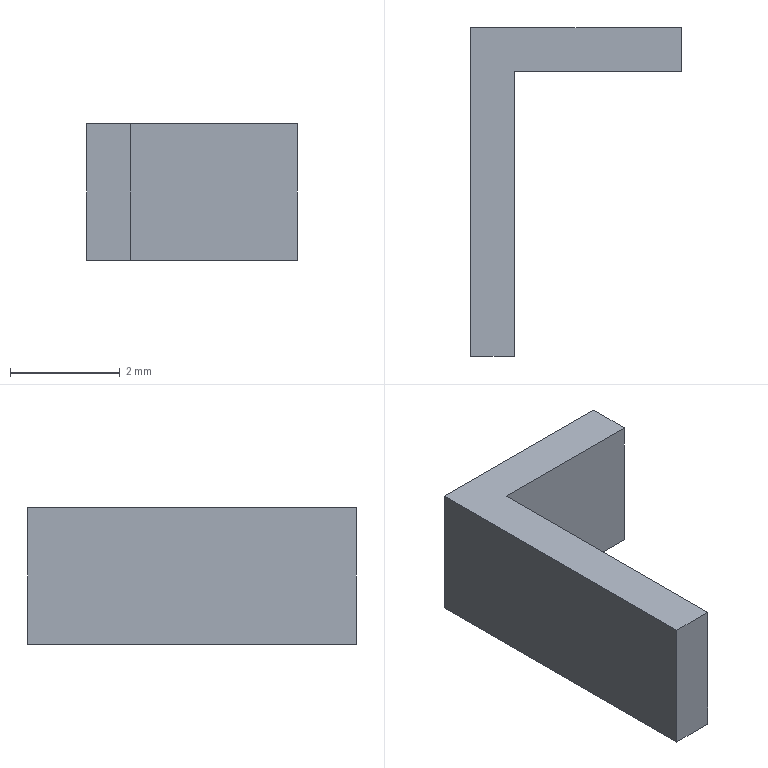Part | STEP file | lll_id1138_x_t | 1 solid | 8 faces | box 3.85 x 6 x 2.5 mm | volume 18.1 mm3 | plane 8
STEP:
#1=CARTESIAN_POINT('',(388.657,-103.274,2.35));
#2=VERTEX_POINT('',#1);
#3=CARTESIAN_POINT('',(387.857,-103.274,2.35));
#4=VERTEX_POINT('',#3);
#5=CARTESIAN_POINT('',(388.257,-103.274,2.35));
#6=DIRECTION('',(-1.,0.,0.));
#7=VECTOR('',#6,1.);
#8=LINE('',#5,#7);
#9=EDGE_CURVE('',#2,#4,#8,.T.);
#10=ORIENTED_EDGE('',*,*,#9,.T.);
#11=CARTESIAN_POINT('',(387.857,-103.274,-0.15));
#12=VERTEX_POINT('',#11);
#13=CARTESIAN_POINT('',(387.857,-103.274,-0.15));
#14=DIRECTION('',(0.,0.,1.));
#15=VECTOR('',#14,1.);
#16=LINE('',#13,#15);
#17=EDGE_CURVE('',#12,#4,#16,.T.);
#18=ORIENTED_EDGE('',*,*,#17,.F.);
#19=CARTESIAN_POINT('',(388.657,-103.274,-0.15));
#20=VERTEX_POINT('',#19);
#21=CARTESIAN_POINT('',(388.257,-103.274,-0.15));
#22=DIRECTION('',(-1.,0.,0.));
#23=VECTOR('',#22,1.);
#24=LINE('',#21,#23);
#25=EDGE_CURVE('',#20,#12,#24,.T.);
#26=ORIENTED_EDGE('',*,*,#25,.F.);
#27=CARTESIAN_POINT('',(388.657,-103.274,-0.15));
#28=DIRECTION('',(0.,0.,1.));
#29=VECTOR('',#28,1.);
#30=LINE('',#27,#29);
#31=EDGE_CURVE('',#20,#2,#30,.T.);
#32=ORIENTED_EDGE('',*,*,#31,.T.);
#33=EDGE_LOOP('',(#10,#18,#26,#32));
#34=FACE_OUTER_BOUND('',#33,.T.);
#35=CARTESIAN_POINT('',(388.657,-103.274,-0.15));
#36=DIRECTION('',(0.,1.,0.));
#37=DIRECTION('',(0.,0.,1.));
#38=AXIS2_PLACEMENT_3D('',#35,#36,#37);
#39=PLANE('',#38);
#40=ADVANCED_FACE('',(#34),#39,.F.);
#41=CARTESIAN_POINT('',(387.857,-97.274,2.35));
#42=VERTEX_POINT('',#41);
#43=CARTESIAN_POINT('',(387.857,-100.274,2.35));
#44=DIRECTION('',(0.,1.,0.));
#45=VECTOR('',#44,1.);
#46=LINE('',#43,#45);
#47=EDGE_CURVE('',#4,#42,#46,.T.);
#48=ORIENTED_EDGE('',*,*,#47,.T.);
#49=CARTESIAN_POINT('',(387.857,-97.274,-0.15));
#50=VERTEX_POINT('',#49);
#51=CARTESIAN_POINT('',(387.857,-97.274,-0.15));
#52=DIRECTION('',(0.,0.,1.));
#53=VECTOR('',#52,1.);
#54=LINE('',#51,#53);
#55=EDGE_CURVE('',#50,#42,#54,.T.);
#56=ORIENTED_EDGE('',*,*,#55,.F.);
#57=CARTESIAN_POINT('',(387.857,-100.274,-0.15));
#58=DIRECTION('',(0.,1.,0.));
#59=VECTOR('',#58,1.);
#60=LINE('',#57,#59);
#61=EDGE_CURVE('',#12,#50,#60,.T.);
#62=ORIENTED_EDGE('',*,*,#61,.F.);
#63=ORIENTED_EDGE('',*,*,#17,.T.);
#64=EDGE_LOOP('',(#48,#56,#62,#63));
#65=FACE_OUTER_BOUND('',#64,.T.);
#66=CARTESIAN_POINT('',(387.857,-103.274,-0.15));
#67=DIRECTION('',(1.,0.,0.));
#68=DIRECTION('',(0.,0.,-1.));
#69=AXIS2_PLACEMENT_3D('',#66,#67,#68);
#70=PLANE('',#69);
#71=ADVANCED_FACE('',(#65),#70,.F.);
#72=CARTESIAN_POINT('',(391.707,-97.274,2.35));
#73=VERTEX_POINT('',#72);
#74=CARTESIAN_POINT('',(389.782,-97.274,2.35));
#75=DIRECTION('',(1.,0.,0.));
#76=VECTOR('',#75,1.);
#77=LINE('',#74,#76);
#78=EDGE_CURVE('',#42,#73,#77,.T.);
#79=ORIENTED_EDGE('',*,*,#78,.T.);
#80=CARTESIAN_POINT('',(391.707,-97.274,-0.15));
#81=VERTEX_POINT('',#80);
#82=CARTESIAN_POINT('',(391.707,-97.274,-0.15));
#83=DIRECTION('',(0.,0.,1.));
#84=VECTOR('',#83,1.);
#85=LINE('',#82,#84);
#86=EDGE_CURVE('',#81,#73,#85,.T.);
#87=ORIENTED_EDGE('',*,*,#86,.F.);
#88=CARTESIAN_POINT('',(389.782,-97.274,-0.15));
#89=DIRECTION('',(1.,0.,0.));
#90=VECTOR('',#89,1.);
#91=LINE('',#88,#90);
#92=EDGE_CURVE('',#50,#81,#91,.T.);
#93=ORIENTED_EDGE('',*,*,#92,.F.);
#94=ORIENTED_EDGE('',*,*,#55,.T.);
#95=EDGE_LOOP('',(#79,#87,#93,#94));
#96=FACE_OUTER_BOUND('',#95,.T.);
#97=CARTESIAN_POINT('',(387.857,-97.274,-0.15));
#98=DIRECTION('',(0.,-1.,0.));
#99=DIRECTION('',(0.,0.,-1.));
#100=AXIS2_PLACEMENT_3D('',#97,#98,#99);
#101=PLANE('',#100);
#102=ADVANCED_FACE('',(#96),#101,.F.);
#103=CARTESIAN_POINT('',(391.707,-98.074,2.35));
#104=VERTEX_POINT('',#103);
#105=CARTESIAN_POINT('',(391.707,-97.674,2.35));
#106=DIRECTION('',(0.,-1.,0.));
#107=VECTOR('',#106,1.);
#108=LINE('',#105,#107);
#109=EDGE_CURVE('',#73,#104,#108,.T.);
#110=ORIENTED_EDGE('',*,*,#109,.T.);
#111=CARTESIAN_POINT('',(391.707,-98.074,-0.15));
#112=VERTEX_POINT('',#111);
#113=CARTESIAN_POINT('',(391.707,-98.074,-0.15));
#114=DIRECTION('',(0.,0.,1.));
#115=VECTOR('',#114,1.);
#116=LINE('',#113,#115);
#117=EDGE_CURVE('',#112,#104,#116,.T.);
#118=ORIENTED_EDGE('',*,*,#117,.F.);
#119=CARTESIAN_POINT('',(391.707,-97.674,-0.15));
#120=DIRECTION('',(0.,-1.,0.));
#121=VECTOR('',#120,1.);
#122=LINE('',#119,#121);
#123=EDGE_CURVE('',#81,#112,#122,.T.);
#124=ORIENTED_EDGE('',*,*,#123,.F.);
#125=ORIENTED_EDGE('',*,*,#86,.T.);
#126=EDGE_LOOP('',(#110,#118,#124,#125));
#127=FACE_OUTER_BOUND('',#126,.T.);
#128=CARTESIAN_POINT('',(391.707,-97.274,-0.15));
#129=DIRECTION('',(-1.,0.,0.));
#130=DIRECTION('',(0.,0.,1.));
#131=AXIS2_PLACEMENT_3D('',#128,#129,#130);
#132=PLANE('',#131);
#133=ADVANCED_FACE('',(#127),#132,.F.);
#134=CARTESIAN_POINT('',(388.657,-98.074,2.35));
#135=VERTEX_POINT('',#134);
#136=CARTESIAN_POINT('',(390.182,-98.074,2.35));
#137=DIRECTION('',(-1.,0.,0.));
#138=VECTOR('',#137,1.);
#139=LINE('',#136,#138);
#140=EDGE_CURVE('',#104,#135,#139,.T.);
#141=ORIENTED_EDGE('',*,*,#140,.T.);
#142=CARTESIAN_POINT('',(388.657,-98.074,-0.15));
#143=VERTEX_POINT('',#142);
#144=CARTESIAN_POINT('',(388.657,-98.074,-0.15));
#145=DIRECTION('',(0.,0.,1.));
#146=VECTOR('',#145,1.);
#147=LINE('',#144,#146);
#148=EDGE_CURVE('',#143,#135,#147,.T.);
#149=ORIENTED_EDGE('',*,*,#148,.F.);
#150=CARTESIAN_POINT('',(390.182,-98.074,-0.15));
#151=DIRECTION('',(-1.,0.,0.));
#152=VECTOR('',#151,1.);
#153=LINE('',#150,#152);
#154=EDGE_CURVE('',#112,#143,#153,.T.);
#155=ORIENTED_EDGE('',*,*,#154,.F.);
#156=ORIENTED_EDGE('',*,*,#117,.T.);
#157=EDGE_LOOP('',(#141,#149,#155,#156));
#158=FACE_OUTER_BOUND('',#157,.T.);
#159=CARTESIAN_POINT('',(391.707,-98.074,-0.15));
#160=DIRECTION('',(0.,1.,0.));
#161=DIRECTION('',(0.,0.,1.));
#162=AXIS2_PLACEMENT_3D('',#159,#160,#161);
#163=PLANE('',#162);
#164=ADVANCED_FACE('',(#158),#163,.F.);
#165=CARTESIAN_POINT('',(388.657,-100.674,2.35));
#166=DIRECTION('',(0.,-1.,0.));
#167=VECTOR('',#166,1.);
#168=LINE('',#165,#167);
#169=EDGE_CURVE('',#135,#2,#168,.T.);
#170=ORIENTED_EDGE('',*,*,#169,.T.);
#171=ORIENTED_EDGE('',*,*,#31,.F.);
#172=CARTESIAN_POINT('',(388.657,-100.674,-0.15));
#173=DIRECTION('',(0.,-1.,0.));
#174=VECTOR('',#173,1.);
#175=LINE('',#172,#174);
#176=EDGE_CURVE('',#143,#20,#175,.T.);
#177=ORIENTED_EDGE('',*,*,#176,.F.);
#178=ORIENTED_EDGE('',*,*,#148,.T.);
#179=EDGE_LOOP('',(#170,#171,#177,#178));
#180=FACE_OUTER_BOUND('',#179,.T.);
#181=CARTESIAN_POINT('',(388.657,-98.074,-0.15));
#182=DIRECTION('',(-1.,0.,0.));
#183=DIRECTION('',(0.,0.,1.));
#184=AXIS2_PLACEMENT_3D('',#181,#182,#183);
#185=PLANE('',#184);
#186=ADVANCED_FACE('',(#180),#185,.F.);
#187=ORIENTED_EDGE('',*,*,#25,.T.);
#188=ORIENTED_EDGE('',*,*,#61,.T.);
#189=ORIENTED_EDGE('',*,*,#92,.T.);
#190=ORIENTED_EDGE('',*,*,#123,.T.);
#191=ORIENTED_EDGE('',*,*,#154,.T.);
#192=ORIENTED_EDGE('',*,*,#176,.T.);
#193=EDGE_LOOP('',(#187,#188,#189,#190,#191,#192));
#194=FACE_OUTER_BOUND('',#193,.T.);
#195=CARTESIAN_POINT('',(388.257,-103.274,-0.15));
#196=DIRECTION('',(0.,0.,1.));
#197=DIRECTION('',(1.,0.,0.));
#198=AXIS2_PLACEMENT_3D('',#195,#196,#197);
#199=PLANE('',#198);
#200=ADVANCED_FACE('',(#194),#199,.F.);
#201=ORIENTED_EDGE('',*,*,#9,.F.);
#202=ORIENTED_EDGE('',*,*,#169,.F.);
#203=ORIENTED_EDGE('',*,*,#140,.F.);
#204=ORIENTED_EDGE('',*,*,#109,.F.);
#205=ORIENTED_EDGE('',*,*,#78,.F.);
#206=ORIENTED_EDGE('',*,*,#47,.F.);
#207=EDGE_LOOP('',(#201,#202,#203,#204,#205,#206));
#208=FACE_OUTER_BOUND('',#207,.T.);
#209=CARTESIAN_POINT('',(388.257,-103.274,2.35));
#210=DIRECTION('',(0.,0.,1.));
#211=DIRECTION('',(1.,0.,0.));
#212=AXIS2_PLACEMENT_3D('',#209,#210,#211);
#213=PLANE('',#212);
#214=ADVANCED_FACE('',(#208),#213,.T.);
#215=CLOSED_SHELL('',(#40,#71,#102,#133,#164,#186,#200,#214));
#216=MANIFOLD_SOLID_BREP('',#215);
#217=(LENGTH_UNIT()NAMED_UNIT(*)SI_UNIT(.MILLI.,.METRE.));
#218=UNCERTAINTY_MEASURE_WITH_UNIT(LENGTH_MEASURE(0.00002),#217,'','');
#219=(NAMED_UNIT(*)PLANE_ANGLE_UNIT()SI_UNIT($,.RADIAN.));
#220=PLANE_ANGLE_MEASURE_WITH_UNIT(PLANE_ANGLE_MEASURE(0.01745),#219);
#221=DIMENSIONAL_EXPONENTS(0.,0.,0.,0.,0.,0.,0.);
#222=(CONVERSION_BASED_UNIT('DEGREE',#220)NAMED_UNIT(#221)PLANE_ANGLE_UNIT());
#223=(NAMED_UNIT(*)SI_UNIT($,.STERADIAN.)SOLID_ANGLE_UNIT());
#224=(GEOMETRIC_REPRESENTATION_CONTEXT(3)GLOBAL_UNCERTAINTY_ASSIGNED_CONTEXT((#218))GLOBAL_UNIT_ASSIGNED_CONTEXT((#217,#222,#223))REPRESENTATION_CONTEXT('',''));
#225=ADVANCED_BREP_SHAPE_REPRESENTATION('',(#216),#224);